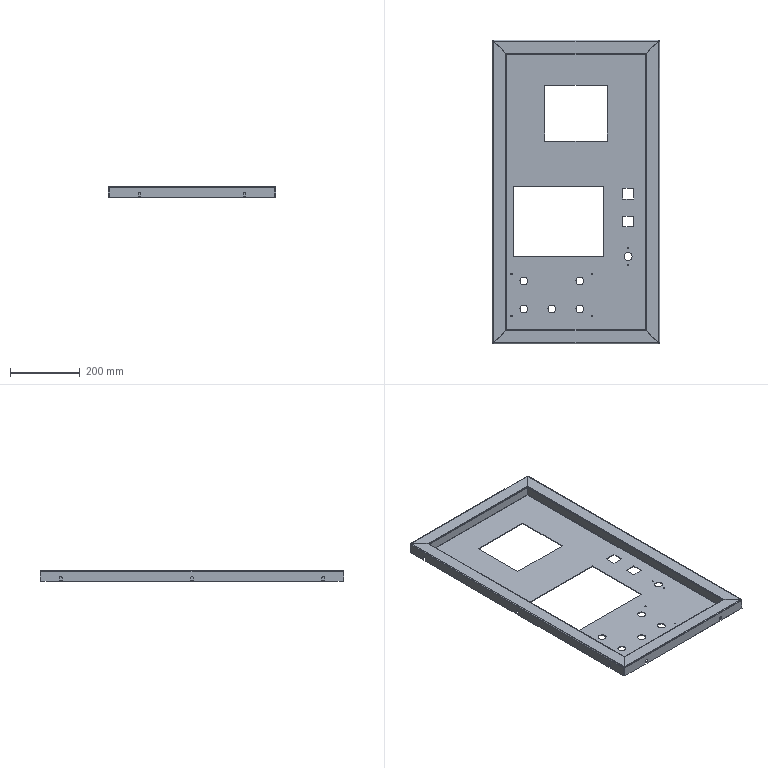Part | NX | 1 solid | 182 faces | box 478 x 869 x 30 mm | volume 930531 mm3 | plane 112 | cylinder 46 | spline 24 | commonest cylinder face diameters 1.473 x12 5.473 x12 7 x10 22.5 x6 4.5 x4 2.5 x2